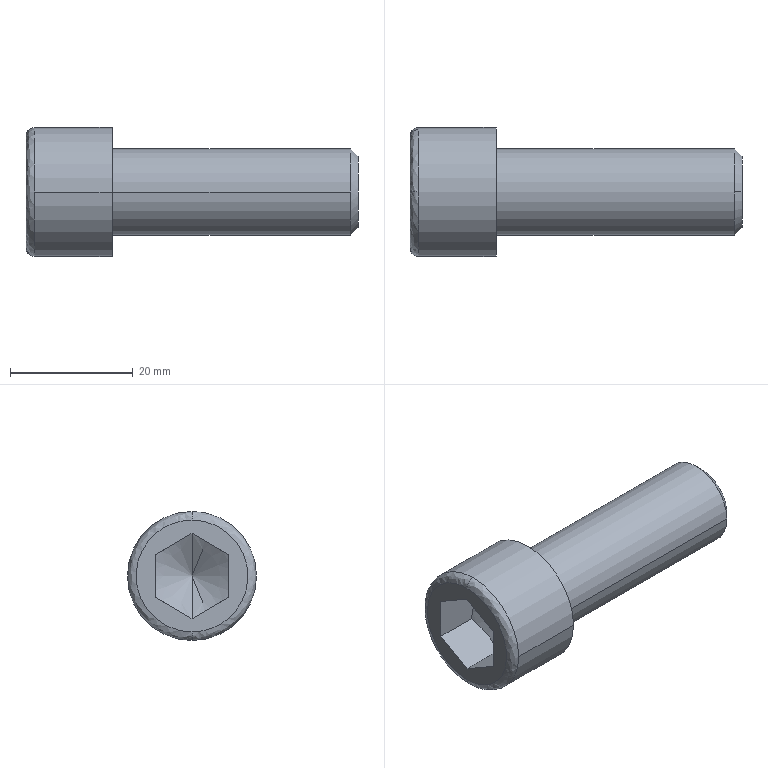Part | STEP file | DIN 912 - replaced by DIN EN ISO 4762 M14 x 40 | 1 solid | 21 faces | box 54 x 21 x 21 mm | volume 9880 mm3 | plane 9 | spline 4 | cylinder 4 | cone 4 | commonest cylinder face diameters 14 x2 21 x2